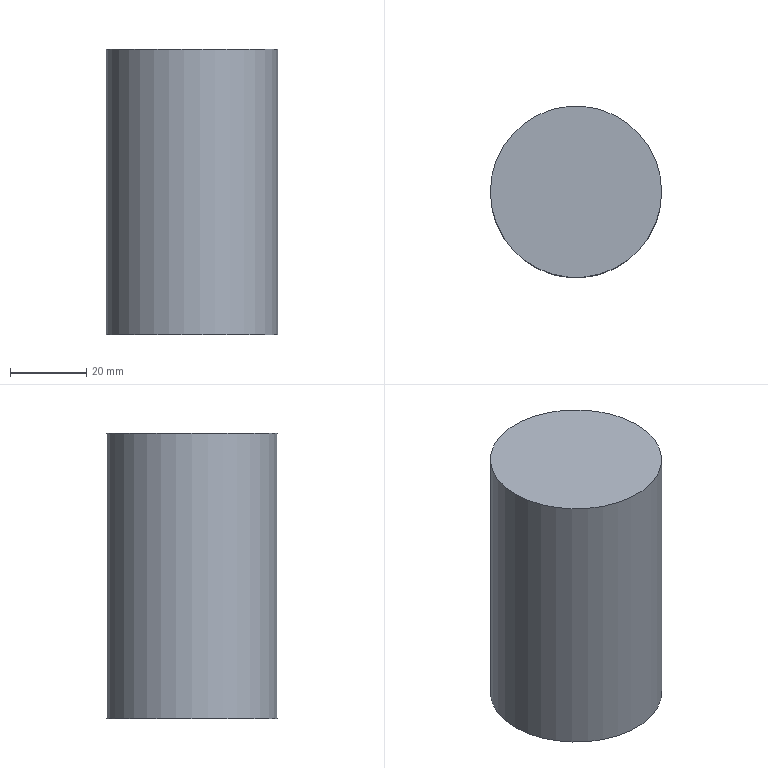Part | NX | features solid 2 | 1 solid | 3 faces | box 45 x 45 x 75 mm | volume 119282 mm3 | plane 2 | cylinder 1 | commonest cylinder face diameters 45 x1
STEP:
#1=CARTESIAN_POINT('',(-552.25,-310.,290.));
#2=VERTEX_POINT('',#1);
#3=CARTESIAN_POINT('',(-574.75,-310.,290.));
#4=DIRECTION('',(0.,0.,-1.));
#5=DIRECTION('',(1.,0.,0.));
#6=AXIS2_PLACEMENT_3D('',#3,#4,#5);
#7=CIRCLE('',#6,22.5);
#8=EDGE_CURVE('',#2,#2,#7,.T.);
#9=ORIENTED_EDGE('',*,*,#8,.T.);
#10=EDGE_LOOP('',(#9));
#11=FACE_BOUND('',#10,.T.);
#12=CARTESIAN_POINT('',(-552.25,-310.,215.));
#13=VERTEX_POINT('',#12);
#14=CARTESIAN_POINT('',(-574.75,-310.,215.));
#15=DIRECTION('',(0.,0.,-1.));
#16=DIRECTION('',(1.,0.,0.));
#17=AXIS2_PLACEMENT_3D('',#14,#15,#16);
#18=CIRCLE('',#17,22.5);
#19=EDGE_CURVE('',#13,#13,#18,.T.);
#20=ORIENTED_EDGE('',*,*,#19,.F.);
#21=EDGE_LOOP('',(#20));
#22=FACE_BOUND('',#21,.T.);
#23=CARTESIAN_POINT('',(-574.75,-310.,290.));
#24=DIRECTION('',(0.,0.,-1.));
#25=DIRECTION('',(-1.,0.,0.));
#26=AXIS2_PLACEMENT_3D('',#23,#24,#25);
#27=CYLINDRICAL_SURFACE('',#26,22.5);
#28=ADVANCED_FACE('',(#11,#22),#27,.T.);
#29=ORIENTED_EDGE('',*,*,#8,.F.);
#30=EDGE_LOOP('',(#29));
#31=FACE_BOUND('',#30,.T.);
#32=CARTESIAN_POINT('',(-574.75,-310.,290.));
#33=DIRECTION('',(0.,0.,1.));
#34=DIRECTION('',(1.,0.,0.));
#35=AXIS2_PLACEMENT_3D('',#32,#33,#34);
#36=PLANE('',#35);
#37=ADVANCED_FACE('',(#31),#36,.T.);
#38=ORIENTED_EDGE('',*,*,#19,.T.);
#39=EDGE_LOOP('',(#38));
#40=FACE_BOUND('',#39,.T.);
#41=CARTESIAN_POINT('',(-574.75,-310.,215.));
#42=DIRECTION('',(0.,0.,1.));
#43=DIRECTION('',(1.,0.,0.));
#44=AXIS2_PLACEMENT_3D('',#41,#42,#43);
#45=PLANE('',#44);
#46=ADVANCED_FACE('',(#40),#45,.F.);
#47=CLOSED_SHELL('',(#28,#37,#46));
#48=MANIFOLD_SOLID_BREP('',#47);
#49=(LENGTH_UNIT()NAMED_UNIT(*)SI_UNIT(.MILLI.,.METRE.));
#50=UNCERTAINTY_MEASURE_WITH_UNIT(LENGTH_MEASURE(0.00001),#49,'','');
#51=(NAMED_UNIT(*)PLANE_ANGLE_UNIT()SI_UNIT($,.RADIAN.));
#52=(NAMED_UNIT(*)SI_UNIT($,.STERADIAN.)SOLID_ANGLE_UNIT());
#53=(GEOMETRIC_REPRESENTATION_CONTEXT(3)GLOBAL_UNCERTAINTY_ASSIGNED_CONTEXT((#50))GLOBAL_UNIT_ASSIGNED_CONTEXT((#49,#51,#52))REPRESENTATION_CONTEXT('',''));
#54=ADVANCED_BREP_SHAPE_REPRESENTATION('',(#48),#53);